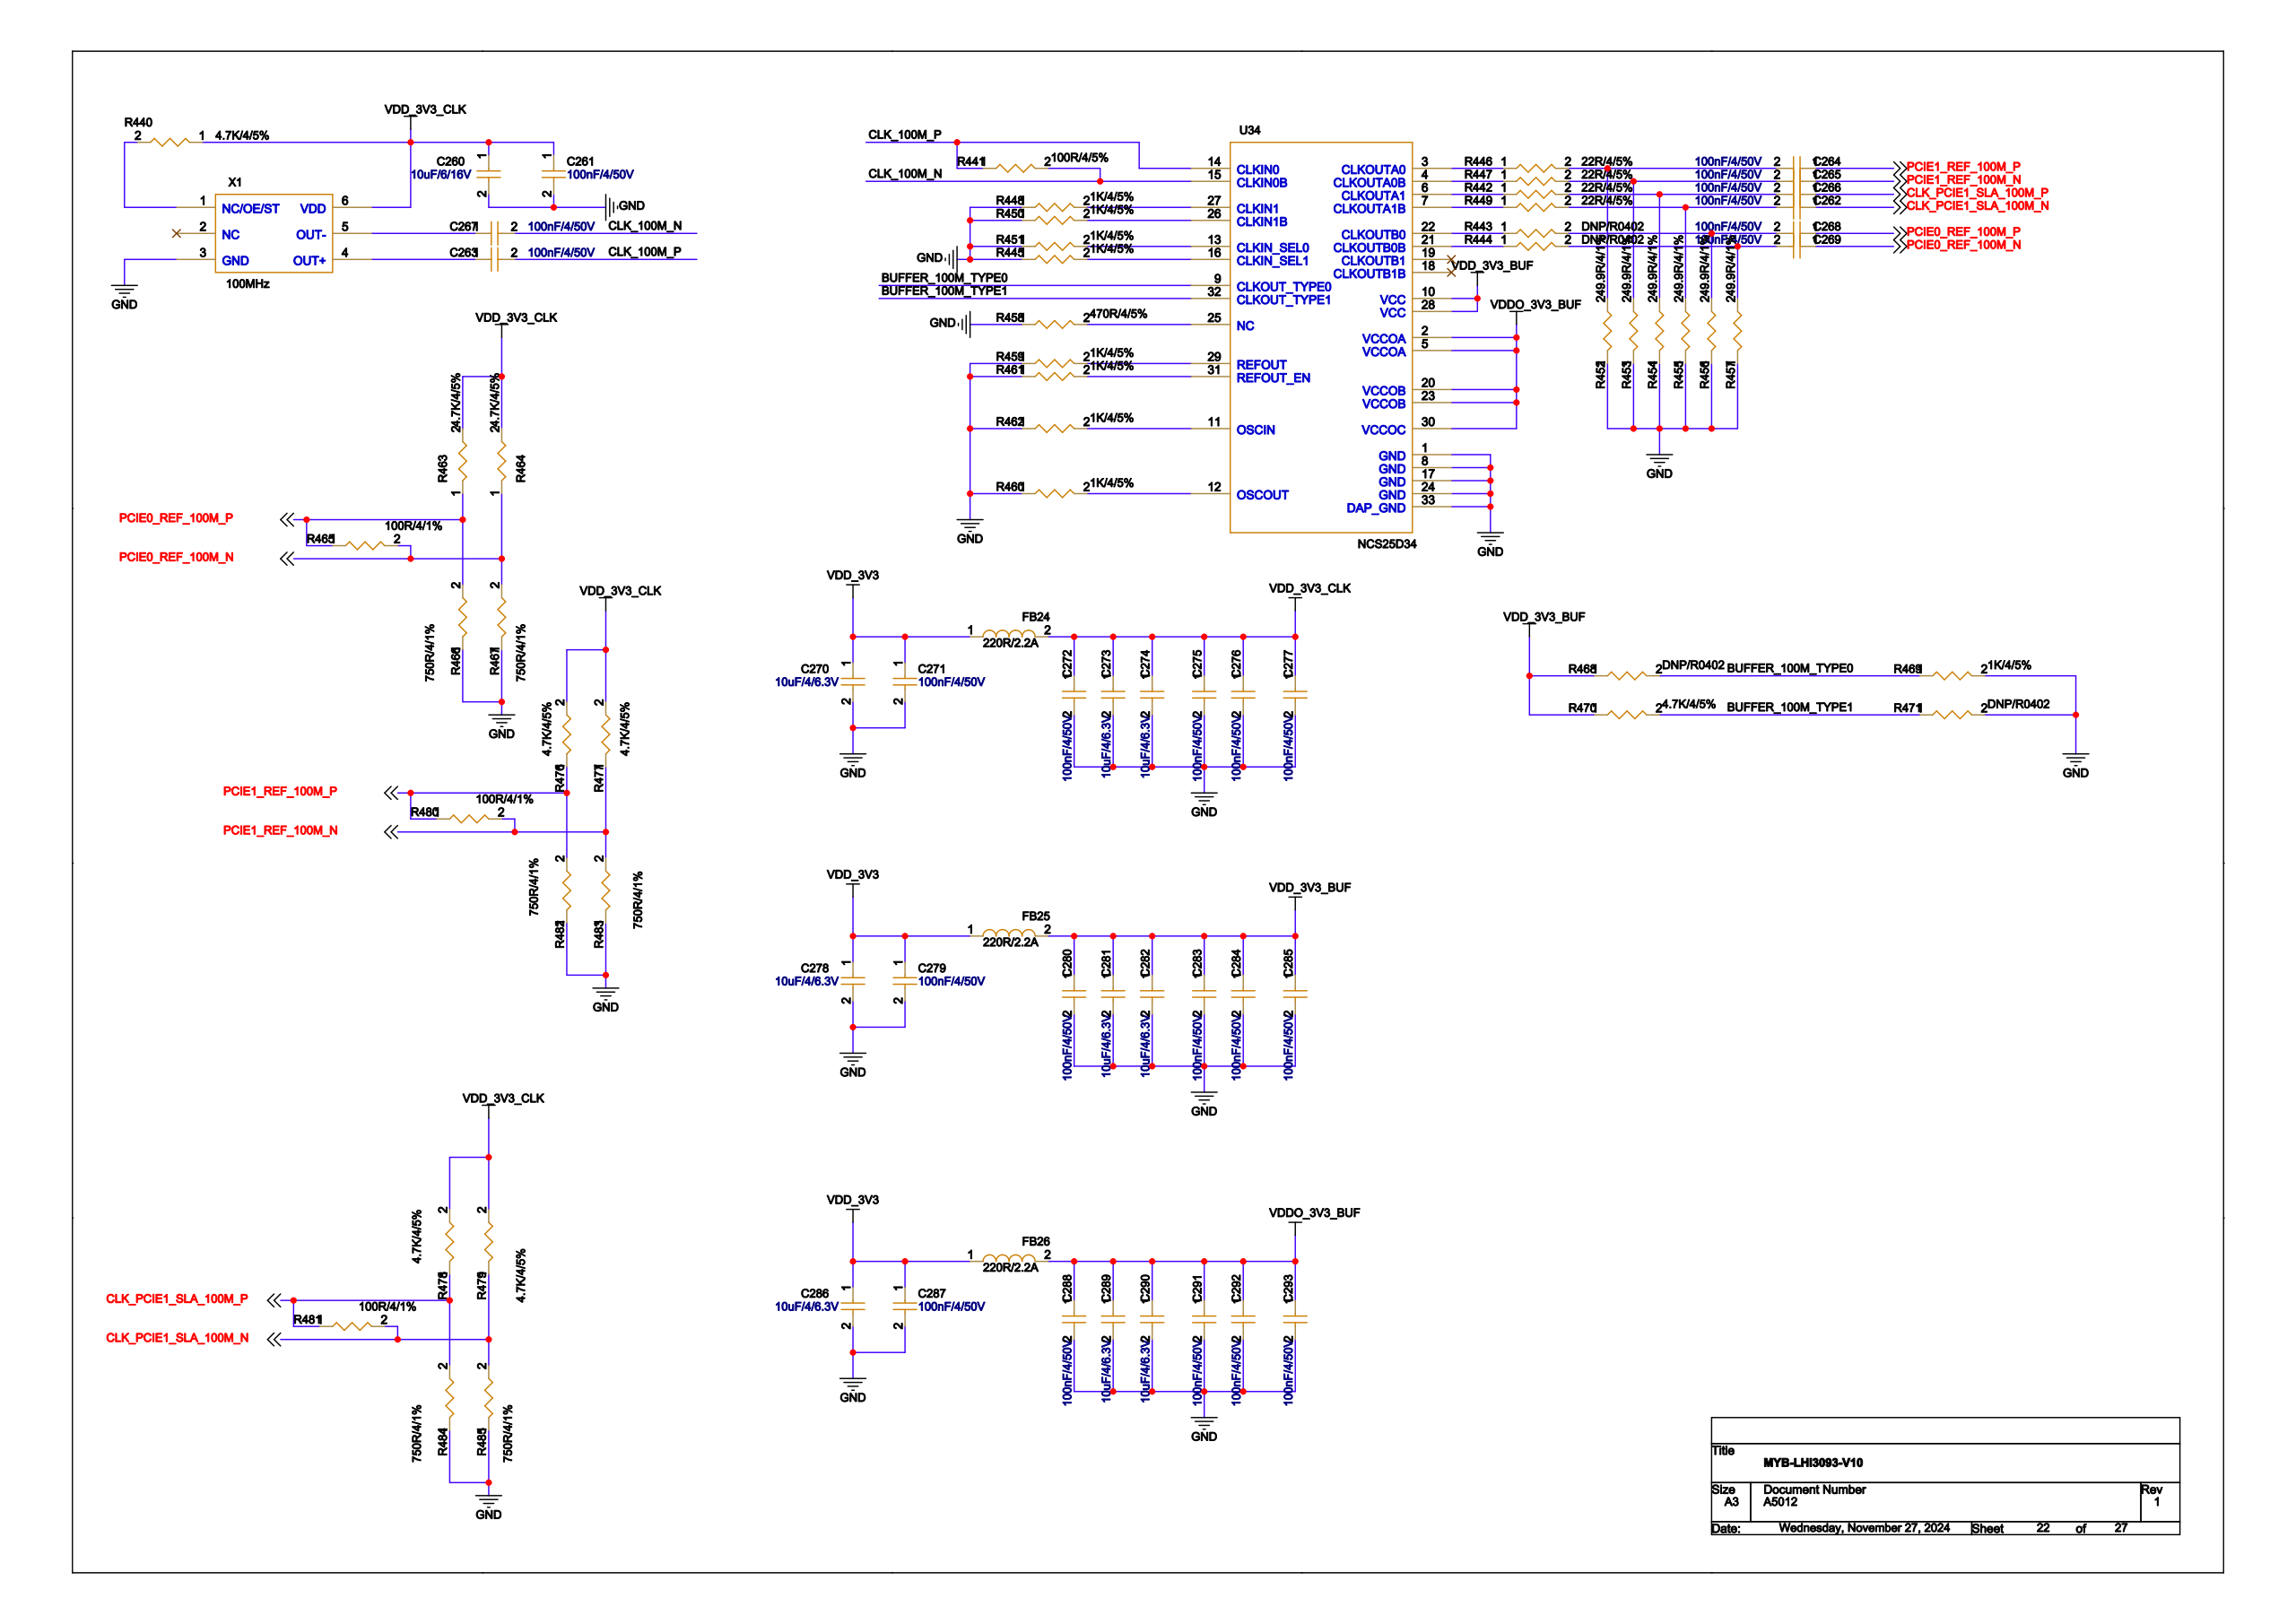Circuit board | Cadence Allegro | 1159 parts | 708 nets | one sheet of the schematic
Parts on this sheet (reference | value | footprint):
C260 | 10uF/6/16V | C0402
C261 | 100nF/4/50V | C0402
C270 | 10uF/4/6.3V | C0402
C271 | 100nF/4/50V | C0402
C272 | 100nF/4/50V | C0402
C273 | 10uF/4/6.3V | C0402
C274 | 10uF/4/6.3V | C0402
C275 | 100nF/4/50V | C0402
C276 | 100nF/4/50V | C0402
C277 | 100nF/4/50V | C0402
C278 | 10uF/4/6.3V | C0402
C279 | 100nF/4/50V | C0402
C280 | 100nF/4/50V | C0402
C281 | 10uF/4/6.3V | C0402
C282 | 10uF/4/6.3V | C0402
C283 | 100nF/4/50V | C0402
C284 | 100nF/4/50V | C0402
C285 | 100nF/4/50V | C0402
C286 | 10uF/4/6.3V | C0402
C287 | 100nF/4/50V | C0402
C288 | 100nF/4/50V | C0402
C289 | 10uF/4/6.3V | C0402
C290 | 10uF/4/6.3V | C0402
C291 | 100nF/4/50V | C0402
C292 | 100nF/4/50V | C0402
C293 | 100nF/4/50V | C0402
FB24 | 220R/2.2A | FB0603
FB25 | 220R/2.2A | FB0603
FB26 | 220R/2.2A | FB0603
R440 | 4.7K/4/5% | R0402
R442 | 22R/4/5% | R0402
R443 | DNP/R0402 | R0402
R444 | DNP/R0402 | R0402
R446 | 22R/4/5% | R0402
R447 | 22R/4/5% | R0402
R449 | 22R/4/5% | R0402
R452 | 49.9R/4/1% | R0402
R453 | 49.9R/4/1% | R0402
R454 | 49.9R/4/1% | R0402
R455 | 49.9R/4/1% | R0402
R456 | 49.9R/4/1% | R0402
R457 | 49.9R/4/1% | R0402
R463 | 4.7K/4/5% | R0402
R464 | 4.7K/4/5% | R0402
R465 | 100R/4/1% | R0402
R466 | 750R/4/1% | R0402
R467 | 750R/4/1% | R0402
R468 | DNP/R0402 | R0402
R471 | DNP/R0402 | R0402
R476 | 4.7K/4/5% | R0402
R477 | 4.7K/4/5% | R0402
R478 | 4.7K/4/5% | R0402
R479 | 4.7K/4/5% | R0402
R480 | 100R/4/1% | R0402
R481 | 100R/4/1% | R0402
R482 | 750R/4/1% | R0402
R484 | 750R/4/1% | R0402
R485 | 750R/4/1% | R0402
U34 | NCS25D34 | QFN32-5X5-0_5
X1 | 100MHz | OSC3225-6
Nets of these parts (net: part-pin ...):
GND: C260-2 C261-2 C270-2 C271-2 C272-2 C273-2 C274-2 C275-2 C276-2 C277-2 C278-2 C279-2 C280-2 C281-2 C282-2 C283-2 C284-2 C285-2 C286-2 C287-2 C288-2 C289-2 C290-2 C291-2 C292-2 C293-2 R452-1 R453-1 R454-1 R455-1 R456-1 R457-1 R466-1 R467-1 R471-2 R482-1 R484-1 R485-1 X1-3 U34-1 U34-8 U34-17 U34-24 U34-33
VDD_3V3: C270-1 C271-1 C278-1 C279-1 C286-1 C287-1 FB24-1 FB25-1 FB26-1
VDD_3V3_CLK: C260-1 C261-1 C272-1 C273-1 C274-1 C275-1 C276-1 C277-1 FB24-2 R440-1 R463-2 R464-2 R476-2 R477-2 R478-2 R479-2 X1-6
CLK_PCIE1_SLA_100M_N: R479-1 R481-2 R485-2
N15063450: R449-2 R455-2
N15060695: X1-4
CLK_100M_P: U34-14
PCIE1_REF_100M_P: R476-1 R480-1 R482-2
N15063141: R446-2 R452-2
PCIE1_REF_100M_N: R477-1 R480-2
N15063254: R447-2 R453-2
CLK_PCIE1_SLA_100M_P: R478-1 R481-1 R484-2
N15063352: R442-2 R454-2
N15060691: X1-5
CLK_100M_N: U34-15
PCIE0_REF_100M_P: R463-1 R465-1 R466-2
N15063548: R443-2 R456-2
PCIE0_REF_100M_N: R464-1 R465-2 R467-2
N15063646: R444-2 R457-2
VDD_3V3_BUF: C280-1 C281-1 C282-1 C283-1 C284-1 C285-1 FB25-2 R468-1 U34-10 U34-28
VDDO_3V3_BUF: C288-1 C289-1 C290-1 C291-1 C292-1 C293-1 FB26-2 U34-2 U34-5 U34-20 U34-23 U34-30
BUFFER_100M_TYPE0: R468-2 U34-9
N15063356: R442-1 U34-6
N15063145: R446-1 U34-3
N15063258: R447-1 U34-4
N15063454: R449-1 U34-7
N15060793: R440-2 X1-1
BUFFER_100M_TYPE1: R471-1 U34-32
N15063552: R443-1 U34-22
N15063650: R444-1 U34-21